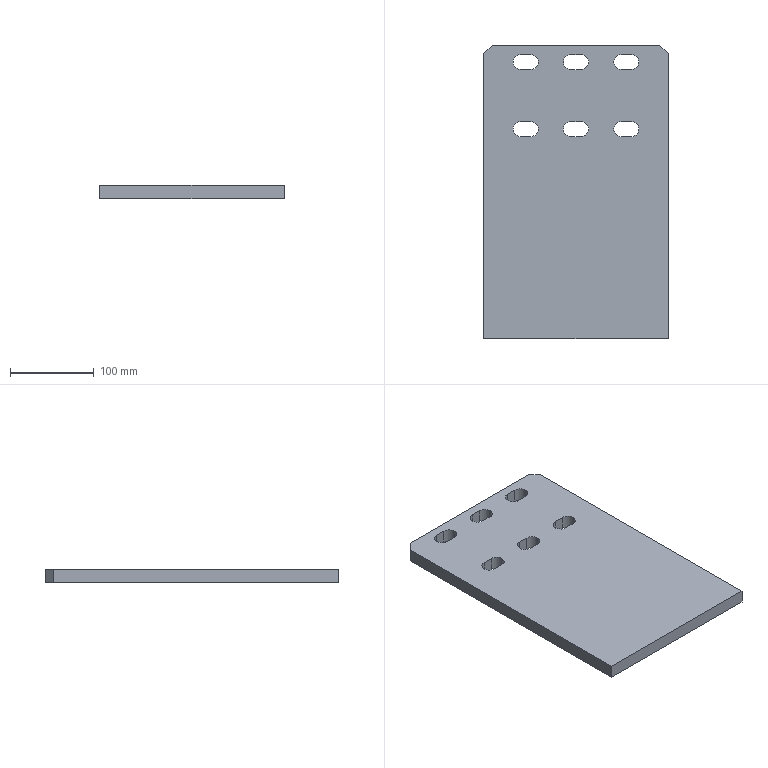Part | STEP file | VD-SYL0380DJ1006_1_1-11_VD-SYL0 | 1 solid | 38 faces | box 220 x 350 x 16 mm | volume 1185235 mm3 | plane 20 | cylinder 18 | commonest cylinder face diameters 18 x18
STEP:
#1=CARTESIAN_POINT('',(66.,66.,0.));
#2=VERTEX_POINT('',#1);
#3=CARTESIAN_POINT('',(75.,75.,0.));
#4=VERTEX_POINT('',#3);
#5=CARTESIAN_POINT('',(66.,75.,0.));
#6=DIRECTION('',(0.,0.,1.));
#7=DIRECTION('',(0.,-1.,0.));
#8=AXIS2_PLACEMENT_3D('',#5,#6,#7);
#9=CIRCLE('',#8,9.);
#10=EDGE_CURVE('',#2,#4,#9,.T.);
#11=ORIENTED_EDGE('',*,*,#10,.F.);
#12=CARTESIAN_POINT('',(66.,66.,16.));
#13=VERTEX_POINT('',#12);
#14=CARTESIAN_POINT('',(66.,66.,0.));
#15=DIRECTION('',(0.,0.,1.));
#16=VECTOR('',#15,1000.);
#17=LINE('',#14,#16);
#18=EDGE_CURVE('',#2,#13,#17,.T.);
#19=ORIENTED_EDGE('',*,*,#18,.T.);
#20=CARTESIAN_POINT('',(75.,75.,16.));
#21=VERTEX_POINT('',#20);
#22=CARTESIAN_POINT('',(66.,75.,16.));
#23=DIRECTION('',(0.,0.,-1.));
#24=DIRECTION('',(1.,0.,0.));
#25=AXIS2_PLACEMENT_3D('',#22,#23,#24);
#26=CIRCLE('',#25,9.);
#27=EDGE_CURVE('',#21,#13,#26,.T.);
#28=ORIENTED_EDGE('',*,*,#27,.F.);
#29=CARTESIAN_POINT('',(75.,75.,16.));
#30=DIRECTION('',(0.,0.,-1.));
#31=VECTOR('',#30,1000.);
#32=LINE('',#29,#31);
#33=EDGE_CURVE('',#21,#4,#32,.T.);
#34=ORIENTED_EDGE('',*,*,#33,.T.);
#35=EDGE_LOOP('',(#11,#19,#28,#34));
#36=FACE_OUTER_BOUND('',#35,.T.);
#37=CARTESIAN_POINT('',(66.,75.,8.));
#38=DIRECTION('',(0.,0.,1.));
#39=DIRECTION('',(1.,0.,0.));
#40=AXIS2_PLACEMENT_3D('',#37,#38,#39);
#41=CYLINDRICAL_SURFACE('',#40,9.);
#42=ADVANCED_FACE('',(#36),#41,.F.);
#43=ORIENTED_EDGE('',*,*,#33,.F.);
#44=CARTESIAN_POINT('',(66.,84.,16.));
#45=VERTEX_POINT('',#44);
#46=CARTESIAN_POINT('',(66.,75.,16.));
#47=DIRECTION('',(0.,0.,-1.));
#48=DIRECTION('',(0.,1.,0.));
#49=AXIS2_PLACEMENT_3D('',#46,#47,#48);
#50=CIRCLE('',#49,9.);
#51=EDGE_CURVE('',#45,#21,#50,.T.);
#52=ORIENTED_EDGE('',*,*,#51,.F.);
#53=CARTESIAN_POINT('',(66.,84.,0.));
#54=VERTEX_POINT('',#53);
#55=CARTESIAN_POINT('',(66.,84.,16.));
#56=DIRECTION('',(0.,0.,-1.));
#57=VECTOR('',#56,1000.);
#58=LINE('',#55,#57);
#59=EDGE_CURVE('',#45,#54,#58,.T.);
#60=ORIENTED_EDGE('',*,*,#59,.T.);
#61=CARTESIAN_POINT('',(66.,75.,0.));
#62=DIRECTION('',(0.,0.,1.));
#63=DIRECTION('',(1.,0.,0.));
#64=AXIS2_PLACEMENT_3D('',#61,#62,#63);
#65=CIRCLE('',#64,9.);
#66=EDGE_CURVE('',#4,#54,#65,.T.);
#67=ORIENTED_EDGE('',*,*,#66,.F.);
#68=EDGE_LOOP('',(#43,#52,#60,#67));
#69=FACE_OUTER_BOUND('',#68,.T.);
#70=CARTESIAN_POINT('',(66.,75.,8.));
#71=DIRECTION('',(0.,0.,1.));
#72=DIRECTION('',(1.,0.,0.));
#73=AXIS2_PLACEMENT_3D('',#70,#71,#72);
#74=CYLINDRICAL_SURFACE('',#73,9.);
#75=ADVANCED_FACE('',(#69),#74,.F.);
#76=CARTESIAN_POINT('',(54.,84.,0.));
#77=VERTEX_POINT('',#76);
#78=CARTESIAN_POINT('',(54.,84.,16.));
#79=VERTEX_POINT('',#78);
#80=CARTESIAN_POINT('',(54.,84.,0.));
#81=DIRECTION('',(0.,0.,1.));
#82=VECTOR('',#81,1000.);
#83=LINE('',#80,#82);
#84=EDGE_CURVE('',#77,#79,#83,.T.);
#85=ORIENTED_EDGE('',*,*,#84,.F.);
#86=CARTESIAN_POINT('',(66.,84.,0.));
#87=DIRECTION('',(-1.,0.,0.));
#88=VECTOR('',#87,1000.);
#89=LINE('',#86,#88);
#90=EDGE_CURVE('',#54,#77,#89,.T.);
#91=ORIENTED_EDGE('',*,*,#90,.F.);
#92=ORIENTED_EDGE('',*,*,#59,.F.);
#93=CARTESIAN_POINT('',(66.,84.,16.));
#94=DIRECTION('',(-1.,0.,0.));
#95=VECTOR('',#94,1000.);
#96=LINE('',#93,#95);
#97=EDGE_CURVE('',#45,#79,#96,.T.);
#98=ORIENTED_EDGE('',*,*,#97,.T.);
#99=EDGE_LOOP('',(#85,#91,#92,#98));
#100=FACE_OUTER_BOUND('',#99,.T.);
#101=CARTESIAN_POINT('',(63.,84.,8.));
#102=DIRECTION('',(0.,1.,0.));
#103=DIRECTION('',(1.,0.,0.));
#104=AXIS2_PLACEMENT_3D('',#101,#102,#103);
#105=PLANE('',#104);
#106=ADVANCED_FACE('',(#100),#105,.F.);
#107=CARTESIAN_POINT('',(54.,66.,16.));
#108=VERTEX_POINT('',#107);
#109=CARTESIAN_POINT('',(54.,75.,16.));
#110=DIRECTION('',(0.,0.,-1.));
#111=DIRECTION('',(-1.,0.,0.));
#112=AXIS2_PLACEMENT_3D('',#109,#110,#111);
#113=CIRCLE('',#112,9.);
#114=EDGE_CURVE('',#108,#79,#113,.T.);
#115=ORIENTED_EDGE('',*,*,#114,.F.);
#116=CARTESIAN_POINT('',(54.,66.,0.));
#117=VERTEX_POINT('',#116);
#118=CARTESIAN_POINT('',(54.,66.,16.));
#119=DIRECTION('',(0.,0.,-1.));
#120=VECTOR('',#119,1000.);
#121=LINE('',#118,#120);
#122=EDGE_CURVE('',#108,#117,#121,.T.);
#123=ORIENTED_EDGE('',*,*,#122,.T.);
#124=CARTESIAN_POINT('',(54.,75.,0.));
#125=DIRECTION('',(0.,0.,1.));
#126=DIRECTION('',(0.,1.,0.));
#127=AXIS2_PLACEMENT_3D('',#124,#125,#126);
#128=CIRCLE('',#127,9.);
#129=EDGE_CURVE('',#77,#117,#128,.T.);
#130=ORIENTED_EDGE('',*,*,#129,.F.);
#131=ORIENTED_EDGE('',*,*,#84,.T.);
#132=EDGE_LOOP('',(#115,#123,#130,#131));
#133=FACE_OUTER_BOUND('',#132,.T.);
#134=CARTESIAN_POINT('',(54.,75.,8.));
#135=DIRECTION('',(0.,0.,1.));
#136=DIRECTION('',(1.,0.,0.));
#137=AXIS2_PLACEMENT_3D('',#134,#135,#136);
#138=CYLINDRICAL_SURFACE('',#137,9.);
#139=ADVANCED_FACE('',(#133),#138,.F.);
#140=ORIENTED_EDGE('',*,*,#18,.F.);
#141=CARTESIAN_POINT('',(54.,66.,0.));
#142=DIRECTION('',(1.,0.,0.));
#143=VECTOR('',#142,1000.);
#144=LINE('',#141,#143);
#145=EDGE_CURVE('',#117,#2,#144,.T.);
#146=ORIENTED_EDGE('',*,*,#145,.F.);
#147=ORIENTED_EDGE('',*,*,#122,.F.);
#148=CARTESIAN_POINT('',(54.,66.,16.));
#149=DIRECTION('',(1.,0.,0.));
#150=VECTOR('',#149,1000.);
#151=LINE('',#148,#150);
#152=EDGE_CURVE('',#108,#13,#151,.T.);
#153=ORIENTED_EDGE('',*,*,#152,.T.);
#154=EDGE_LOOP('',(#140,#146,#147,#153));
#155=FACE_OUTER_BOUND('',#154,.T.);
#156=CARTESIAN_POINT('',(57.,66.,8.));
#157=DIRECTION('',(0.,-1.,0.));
#158=DIRECTION('',(0.,0.,-1.));
#159=AXIS2_PLACEMENT_3D('',#156,#157,#158);
#160=PLANE('',#159);
#161=ADVANCED_FACE('',(#155),#160,.F.);
#162=CARTESIAN_POINT('',(-6.,84.,0.));
#163=VERTEX_POINT('',#162);
#164=CARTESIAN_POINT('',(-6.,84.,16.));
#165=VERTEX_POINT('',#164);
#166=CARTESIAN_POINT('',(-6.,84.,0.));
#167=DIRECTION('',(0.,0.,1.));
#168=VECTOR('',#167,1000.);
#169=LINE('',#166,#168);
#170=EDGE_CURVE('',#163,#165,#169,.T.);
#171=ORIENTED_EDGE('',*,*,#170,.F.);
#172=CARTESIAN_POINT('',(6.,84.,0.));
#173=VERTEX_POINT('',#172);
#174=CARTESIAN_POINT('',(6.,84.,0.));
#175=DIRECTION('',(-1.,0.,0.));
#176=VECTOR('',#175,1000.);
#177=LINE('',#174,#176);
#178=EDGE_CURVE('',#173,#163,#177,.T.);
#179=ORIENTED_EDGE('',*,*,#178,.F.);
#180=CARTESIAN_POINT('',(6.,84.,16.));
#181=VERTEX_POINT('',#180);
#182=CARTESIAN_POINT('',(6.,84.,16.));
#183=DIRECTION('',(0.,0.,-1.));
#184=VECTOR('',#183,1000.);
#185=LINE('',#182,#184);
#186=EDGE_CURVE('',#181,#173,#185,.T.);
#187=ORIENTED_EDGE('',*,*,#186,.F.);
#188=CARTESIAN_POINT('',(6.,84.,16.));
#189=DIRECTION('',(-1.,0.,0.));
#190=VECTOR('',#189,1000.);
#191=LINE('',#188,#190);
#192=EDGE_CURVE('',#181,#165,#191,.T.);
#193=ORIENTED_EDGE('',*,*,#192,.T.);
#194=EDGE_LOOP('',(#171,#179,#187,#193));
#195=FACE_OUTER_BOUND('',#194,.T.);
#196=CARTESIAN_POINT('',(3.,84.,8.));
#197=DIRECTION('',(0.,1.,0.));
#198=DIRECTION('',(1.,0.,0.));
#199=AXIS2_PLACEMENT_3D('',#196,#197,#198);
#200=PLANE('',#199);
#201=ADVANCED_FACE('',(#195),#200,.F.);
#202=CARTESIAN_POINT('',(15.,75.,16.));
#203=VERTEX_POINT('',#202);
#204=CARTESIAN_POINT('',(15.,75.,0.));
#205=VERTEX_POINT('',#204);
#206=CARTESIAN_POINT('',(15.,75.,16.));
#207=DIRECTION('',(0.,0.,-1.));
#208=VECTOR('',#207,1000.);
#209=LINE('',#206,#208);
#210=EDGE_CURVE('',#203,#205,#209,.T.);
#211=ORIENTED_EDGE('',*,*,#210,.F.);
#212=CARTESIAN_POINT('',(6.,75.,16.));
#213=DIRECTION('',(0.,0.,-1.));
#214=DIRECTION('',(0.,1.,0.));
#215=AXIS2_PLACEMENT_3D('',#212,#213,#214);
#216=CIRCLE('',#215,9.);
#217=EDGE_CURVE('',#181,#203,#216,.T.);
#218=ORIENTED_EDGE('',*,*,#217,.F.);
#219=ORIENTED_EDGE('',*,*,#186,.T.);
#220=CARTESIAN_POINT('',(6.,75.,0.));
#221=DIRECTION('',(0.,0.,1.));
#222=DIRECTION('',(1.,0.,0.));
#223=AXIS2_PLACEMENT_3D('',#220,#221,#222);
#224=CIRCLE('',#223,9.);
#225=EDGE_CURVE('',#205,#173,#224,.T.);
#226=ORIENTED_EDGE('',*,*,#225,.F.);
#227=EDGE_LOOP('',(#211,#218,#219,#226));
#228=FACE_OUTER_BOUND('',#227,.T.);
#229=CARTESIAN_POINT('',(6.,75.,8.));
#230=DIRECTION('',(0.,0.,1.));
#231=DIRECTION('',(1.,0.,0.));
#232=AXIS2_PLACEMENT_3D('',#229,#230,#231);
#233=CYLINDRICAL_SURFACE('',#232,9.);
#234=ADVANCED_FACE('',(#228),#233,.F.);
#235=CARTESIAN_POINT('',(6.,66.,0.));
#236=VERTEX_POINT('',#235);
#237=CARTESIAN_POINT('',(6.,75.,0.));
#238=DIRECTION('',(0.,0.,1.));
#239=DIRECTION('',(0.,-1.,0.));
#240=AXIS2_PLACEMENT_3D('',#237,#238,#239);
#241=CIRCLE('',#240,9.);
#242=EDGE_CURVE('',#236,#205,#241,.T.);
#243=ORIENTED_EDGE('',*,*,#242,.F.);
#244=CARTESIAN_POINT('',(6.,66.,16.));
#245=VERTEX_POINT('',#244);
#246=CARTESIAN_POINT('',(6.,66.,0.));
#247=DIRECTION('',(0.,0.,1.));
#248=VECTOR('',#247,1000.);
#249=LINE('',#246,#248);
#250=EDGE_CURVE('',#236,#245,#249,.T.);
#251=ORIENTED_EDGE('',*,*,#250,.T.);
#252=CARTESIAN_POINT('',(6.,75.,16.));
#253=DIRECTION('',(0.,0.,-1.));
#254=DIRECTION('',(1.,0.,0.));
#255=AXIS2_PLACEMENT_3D('',#252,#253,#254);
#256=CIRCLE('',#255,9.);
#257=EDGE_CURVE('',#203,#245,#256,.T.);
#258=ORIENTED_EDGE('',*,*,#257,.F.);
#259=ORIENTED_EDGE('',*,*,#210,.T.);
#260=EDGE_LOOP('',(#243,#251,#258,#259));
#261=FACE_OUTER_BOUND('',#260,.T.);
#262=CARTESIAN_POINT('',(6.,75.,8.));
#263=DIRECTION('',(0.,0.,1.));
#264=DIRECTION('',(1.,0.,0.));
#265=AXIS2_PLACEMENT_3D('',#262,#263,#264);
#266=CYLINDRICAL_SURFACE('',#265,9.);
#267=ADVANCED_FACE('',(#261),#266,.F.);
#268=ORIENTED_EDGE('',*,*,#250,.F.);
#269=CARTESIAN_POINT('',(-6.,66.,0.));
#270=VERTEX_POINT('',#269);
#271=CARTESIAN_POINT('',(-6.,66.,0.));
#272=DIRECTION('',(1.,0.,0.));
#273=VECTOR('',#272,1000.);
#274=LINE('',#271,#273);
#275=EDGE_CURVE('',#270,#236,#274,.T.);
#276=ORIENTED_EDGE('',*,*,#275,.F.);
#277=CARTESIAN_POINT('',(-6.,66.,16.));
#278=VERTEX_POINT('',#277);
#279=CARTESIAN_POINT('',(-6.,66.,16.));
#280=DIRECTION('',(0.,0.,-1.));
#281=VECTOR('',#280,1000.);
#282=LINE('',#279,#281);
#283=EDGE_CURVE('',#278,#270,#282,.T.);
#284=ORIENTED_EDGE('',*,*,#283,.F.);
#285=CARTESIAN_POINT('',(-6.,66.,16.));
#286=DIRECTION('',(1.,0.,0.));
#287=VECTOR('',#286,1000.);
#288=LINE('',#285,#287);
#289=EDGE_CURVE('',#278,#245,#288,.T.);
#290=ORIENTED_EDGE('',*,*,#289,.T.);
#291=EDGE_LOOP('',(#268,#276,#284,#290));
#292=FACE_OUTER_BOUND('',#291,.T.);
#293=CARTESIAN_POINT('',(-3.,66.,8.));
#294=DIRECTION('',(0.,-1.,0.));
#295=DIRECTION('',(0.,0.,-1.));
#296=AXIS2_PLACEMENT_3D('',#293,#294,#295);
#297=PLANE('',#296);
#298=ADVANCED_FACE('',(#292),#297,.F.);
#299=CARTESIAN_POINT('',(-54.,66.,0.));
#300=VERTEX_POINT('',#299);
#301=CARTESIAN_POINT('',(-45.,75.,0.));
#302=VERTEX_POINT('',#301);
#303=CARTESIAN_POINT('',(-54.,75.,0.));
#304=DIRECTION('',(0.,0.,1.));
#305=DIRECTION('',(0.,-1.,0.));
#306=AXIS2_PLACEMENT_3D('',#303,#304,#305);
#307=CIRCLE('',#306,9.);
#308=EDGE_CURVE('',#300,#302,#307,.T.);
#309=ORIENTED_EDGE('',*,*,#308,.F.);
#310=CARTESIAN_POINT('',(-54.,66.,16.));
#311=VERTEX_POINT('',#310);
#312=CARTESIAN_POINT('',(-54.,66.,0.));
#313=DIRECTION('',(0.,0.,1.));
#314=VECTOR('',#313,1000.);
#315=LINE('',#312,#314);
#316=EDGE_CURVE('',#300,#311,#315,.T.);
#317=ORIENTED_EDGE('',*,*,#316,.T.);
#318=CARTESIAN_POINT('',(-45.,75.,16.));
#319=VERTEX_POINT('',#318);
#320=CARTESIAN_POINT('',(-54.,75.,16.));
#321=DIRECTION('',(0.,0.,-1.));
#322=DIRECTION('',(1.,0.,0.));
#323=AXIS2_PLACEMENT_3D('',#320,#321,#322);
#324=CIRCLE('',#323,9.);
#325=EDGE_CURVE('',#319,#311,#324,.T.);
#326=ORIENTED_EDGE('',*,*,#325,.F.);
#327=CARTESIAN_POINT('',(-45.,75.,16.));
#328=DIRECTION('',(0.,0.,-1.));
#329=VECTOR('',#328,1000.);
#330=LINE('',#327,#329);
#331=EDGE_CURVE('',#319,#302,#330,.T.);
#332=ORIENTED_EDGE('',*,*,#331,.T.);
#333=EDGE_LOOP('',(#309,#317,#326,#332));
#334=FACE_OUTER_BOUND('',#333,.T.);
#335=CARTESIAN_POINT('',(-54.,75.,8.));
#336=DIRECTION('',(0.,0.,1.));
#337=DIRECTION('',(1.,0.,0.));
#338=AXIS2_PLACEMENT_3D('',#335,#336,#337);
#339=CYLINDRICAL_SURFACE('',#338,9.);
#340=ADVANCED_FACE('',(#334),#339,.F.);
#341=ORIENTED_EDGE('',*,*,#331,.F.);
#342=CARTESIAN_POINT('',(-54.,84.,16.));
#343=VERTEX_POINT('',#342);
#344=CARTESIAN_POINT('',(-54.,75.,16.));
#345=DIRECTION('',(0.,0.,-1.));
#346=DIRECTION('',(0.,1.,0.));
#347=AXIS2_PLACEMENT_3D('',#344,#345,#346);
#348=CIRCLE('',#347,9.);
#349=EDGE_CURVE('',#343,#319,#348,.T.);
#350=ORIENTED_EDGE('',*,*,#349,.F.);
#351=CARTESIAN_POINT('',(-54.,84.,0.));
#352=VERTEX_POINT('',#351);
#353=CARTESIAN_POINT('',(-54.,84.,16.));
#354=DIRECTION('',(0.,0.,-1.));
#355=VECTOR('',#354,1000.);
#356=LINE('',#353,#355);
#357=EDGE_CURVE('',#343,#352,#356,.T.);
#358=ORIENTED_EDGE('',*,*,#357,.T.);
#359=CARTESIAN_POINT('',(-54.,75.,0.));
#360=DIRECTION('',(0.,0.,1.));
#361=DIRECTION('',(1.,0.,0.));
#362=AXIS2_PLACEMENT_3D('',#359,#360,#361);
#363=CIRCLE('',#362,9.);
#364=EDGE_CURVE('',#302,#352,#363,.T.);
#365=ORIENTED_EDGE('',*,*,#364,.F.);
#366=EDGE_LOOP('',(#341,#350,#358,#365));
#367=FACE_OUTER_BOUND('',#366,.T.);
#368=CARTESIAN_POINT('',(-54.,75.,8.));
#369=DIRECTION('',(0.,0.,1.));
#370=DIRECTION('',(1.,0.,0.));
#371=AXIS2_PLACEMENT_3D('',#368,#369,#370);
#372=CYLINDRICAL_SURFACE('',#371,9.);
#373=ADVANCED_FACE('',(#367),#372,.F.);
#374=CARTESIAN_POINT('',(-66.,84.,0.));
#375=VERTEX_POINT('',#374);
#376=CARTESIAN_POINT('',(-66.,84.,16.));
#377=VERTEX_POINT('',#376);
#378=CARTESIAN_POINT('',(-66.,84.,0.));
#379=DIRECTION('',(0.,0.,1.));
#380=VECTOR('',#379,1000.);
#381=LINE('',#378,#380);
#382=EDGE_CURVE('',#375,#377,#381,.T.);
#383=ORIENTED_EDGE('',*,*,#382,.F.);
#384=CARTESIAN_POINT('',(-54.,84.,0.));
#385=DIRECTION('',(-1.,0.,0.));
#386=VECTOR('',#385,1000.);
#387=LINE('',#384,#386);
#388=EDGE_CURVE('',#352,#375,#387,.T.);
#389=ORIENTED_EDGE('',*,*,#388,.F.);
#390=ORIENTED_EDGE('',*,*,#357,.F.);
#391=CARTESIAN_POINT('',(-54.,84.,16.));
#392=DIRECTION('',(-1.,0.,0.));
#393=VECTOR('',#392,1000.);
#394=LINE('',#391,#393);
#395=EDGE_CURVE('',#343,#377,#394,.T.);
#396=ORIENTED_EDGE('',*,*,#395,.T.);
#397=EDGE_LOOP('',(#383,#389,#390,#396));
#398=FACE_OUTER_BOUND('',#397,.T.);
#399=CARTESIAN_POINT('',(-57.,84.,8.));
#400=DIRECTION('',(0.,1.,0.));
#401=DIRECTION('',(1.,0.,0.));
#402=AXIS2_PLACEMENT_3D('',#399,#400,#401);
#403=PLANE('',#402);
#404=ADVANCED_FACE('',(#398),#403,.F.);
#405=CARTESIAN_POINT('',(-66.,66.,16.));
#406=VERTEX_POINT('',#405);
#407=CARTESIAN_POINT('',(-66.,75.,16.));
#408=DIRECTION('',(0.,0.,-1.));
#409=DIRECTION('',(-1.,0.,0.));
#410=AXIS2_PLACEMENT_3D('',#407,#408,#409);
#411=CIRCLE('',#410,9.);
#412=EDGE_CURVE('',#406,#377,#411,.T.);
#413=ORIENTED_EDGE('',*,*,#412,.F.);
#414=CARTESIAN_POINT('',(-66.,66.,0.));
#415=VERTEX_POINT('',#414);
#416=CARTESIAN_POINT('',(-66.,66.,16.));
#417=DIRECTION('',(0.,0.,-1.));
#418=VECTOR('',#417,1000.);
#419=LINE('',#416,#418);
#420=EDGE_CURVE('',#406,#415,#419,.T.);
#421=ORIENTED_EDGE('',*,*,#420,.T.);
#422=CARTESIAN_POINT('',(-66.,75.,0.));
#423=DIRECTION('',(0.,0.,1.));
#424=DIRECTION('',(0.,1.,0.));
#425=AXIS2_PLACEMENT_3D('',#422,#423,#424);
#426=CIRCLE('',#425,9.);
#427=EDGE_CURVE('',#375,#415,#426,.T.);
#428=ORIENTED_EDGE('',*,*,#427,.F.);
#429=ORIENTED_EDGE('',*,*,#382,.T.);
#430=EDGE_LOOP('',(#413,#421,#428,#429));
#431=FACE_OUTER_BOUND('',#430,.T.);
#432=CARTESIAN_POINT('',(-66.,75.,8.));
#433=DIRECTION('',(0.,0.,1.));
#434=DIRECTION('',(1.,0.,0.));
#435=AXIS2_PLACEMENT_3D('',#432,#433,#434);
#436=CYLINDRICAL_SURFACE('',#435,9.);
#437=ADVANCED_FACE('',(#431),#436,.F.);
#438=ORIENTED_EDGE('',*,*,#316,.F.);
#439=CARTESIAN_POINT('',(-66.,66.,0.));
#440=DIRECTION('',(1.,0.,0.));
#441=VECTOR('',#440,1000.);
#442=LINE('',#439,#441);
#443=EDGE_CURVE('',#415,#300,#442,.T.);
#444=ORIENTED_EDGE('',*,*,#443,.F.);
#445=ORIENTED_EDGE('',*,*,#420,.F.);
#446=CARTESIAN_POINT('',(-66.,66.,16.));
#447=DIRECTION('',(1.,0.,0.));
#448=VECTOR('',#447,1000.);
#449=LINE('',#446,#448);
#450=EDGE_CURVE('',#406,#311,#449,.T.);
#451=ORIENTED_EDGE('',*,*,#450,.T.);
#452=EDGE_LOOP('',(#438,#444,#445,#451));
#453=FACE_OUTER_BOUND('',#452,.T.);
#454=CARTESIAN_POINT('',(-63.,66.,8.));
#455=DIRECTION('',(0.,-1.,0.));
#456=DIRECTION('',(0.,0.,-1.));
#457=AXIS2_PLACEMENT_3D('',#454,#455,#456);
#458=PLANE('',#457);
#459=ADVANCED_FACE('',(#453),#458,.F.);
#460=CARTESIAN_POINT('',(66.,146.,0.));
#461=VERTEX_POINT('',#460);
#462=CARTESIAN_POINT('',(75.,155.,0.));
#463=VERTEX_POINT('',#462);
#464=CARTESIAN_POINT('',(66.,155.,0.));
#465=DIRECTION('',(0.,0.,1.));
#466=DIRECTION('',(0.,-1.,0.));
#467=AXIS2_PLACEMENT_3D('',#464,#465,#466);
#468=CIRCLE('',#467,9.);
#469=EDGE_CURVE('',#461,#463,#468,.T.);
#470=ORIENTED_EDGE('',*,*,#469,.F.);
#471=CARTESIAN_POINT('',(66.,146.,16.));
#472=VERTEX_POINT('',#471);
#473=CARTESIAN_POINT('',(66.,146.,0.));
#474=DIRECTION('',(0.,0.,1.));
#475=VECTOR('',#474,1000.);
#476=LINE('',#473,#475);
#477=EDGE_CURVE('',#461,#472,#476,.T.);
#478=ORIENTED_EDGE('',*,*,#477,.T.);
#479=CARTESIAN_POINT('',(75.,155.,16.));
#480=VERTEX_POINT('',#479);
#481=CARTESIAN_POINT('',(66.,155.,16.));
#482=DIRECTION('',(0.,0.,-1.));
#483=DIRECTION('',(1.,0.,0.));
#484=AXIS2_PLACEMENT_3D('',#481,#482,#483);
#485=CIRCLE('',#484,9.);
#486=EDGE_CURVE('',#480,#472,#485,.T.);
#487=ORIENTED_EDGE('',*,*,#486,.F.);
#488=CARTESIAN_POINT('',(75.,155.,16.));
#489=DIRECTION('',(0.,0.,-1.));
#490=VECTOR('',#489,1000.);
#491=LINE('',#488,#490);
#492=EDGE_CURVE('',#480,#463,#491,.T.);
#493=ORIENTED_EDGE('',*,*,#492,.T.);
#494=EDGE_LOOP('',(#470,#478,#487,#493));
#495=FACE_OUTER_BOUND('',#494,.T.);
#496=CARTESIAN_POINT('',(66.,155.,8.));
#497=DIRECTION('',(0.,0.,1.));
#498=DIRECTION('',(1.,0.,0.));
#499=AXIS2_PLACEMENT_3D('',#496,#497,#498);
#500=CYLINDRICAL_SURFACE('',#499,9.);
#501=ADVANCED_FACE('',(#495),#500,.F.);
#502=ORIENTED_EDGE('',*,*,#492,.F.);
#503=CARTESIAN_POINT('',(66.,164.,16.));
#504=VERTEX_POINT('',#503);
#505=CARTESIAN_POINT('',(66.,155.,16.));
#506=DIRECTION('',(0.,0.,-1.));
#507=DIRECTION('',(0.,1.,0.));
#508=AXIS2_PLACEMENT_3D('',#505,#506,#507);
#509=CIRCLE('',#508,9.);
#510=EDGE_CURVE('',#504,#480,#509,.T.);
#511=ORIENTED_EDGE('',*,*,#510,.F.);
#512=CARTESIAN_POINT('',(66.,164.,0.));
#513=VERTEX_POINT('',#512);
#514=CARTESIAN_POINT('',(66.,164.,16.));
#515=DIRECTION('',(0.,0.,-1.));
#516=VECTOR('',#515,1000.);
#517=LINE('',#514,#516);
#518=EDGE_CURVE('',#504,#513,#517,.T.);
#519=ORIENTED_EDGE('',*,*,#518,.T.);
#520=CARTESIAN_POINT('',(66.,155.,0.));
#521=DIRECTION('',(0.,0.,1.));
#522=DIRECTION('',(1.,0.,0.));
#523=AXIS2_PLACEMENT_3D('',#520,#521,#522);
#524=CIRCLE('',#523,9.);
#525=EDGE_CURVE('',#463,#513,#524,.T.);
#526=ORIENTED_EDGE('',*,*,#525,.F.);
#527=EDGE_LOOP('',(#502,#511,#519,#526));
#528=FACE_OUTER_BOUND('',#527,.T.);
#529=CARTESIAN_POINT('',(66.,155.,8.));
#530=DIRECTION('',(0.,0.,1.));
#531=DIRECTION('',(1.,0.,0.));
#532=AXIS2_PLACEMENT_3D('',#529,#530,#531);
#533=CYLINDRICAL_SURFACE('',#532,9.);
#534=ADVANCED_FACE('',(#528),#533,.F.);
#535=CARTESIAN_POINT('',(54.,164.,0.));
#536=VERTEX_POINT('',#535);
#537=CARTESIAN_POINT('',(54.,164.,16.));
#538=VERTEX_POINT('',#537);
#539=CARTESIAN_POINT('',(54.,164.,0.));
#540=DIRECTION('',(0.,0.,1.));
#541=VECTOR('',#540,1000.);
#542=LINE('',#539,#541);
#543=EDGE_CURVE('',#536,#538,#542,.T.);
#544=ORIENTED_EDGE('',*,*,#543,.F.);
#545=CARTESIAN_POINT('',(66.,164.,0.));
#546=DIRECTION('',(-1.,0.,0.));
#547=VECTOR('',#546,1000.);
#548=LINE('',#545,#547);
#549=EDGE_CURVE('',#513,#536,#548,.T.);
#550=ORIENTED_EDGE('',*,*,#549,.F.);
#551=ORIENTED_EDGE('',*,*,#518,.F.);
#552=CARTESIAN_POINT('',(66.,164.,16.));
#553=DIRECTION('',(-1.,0.,0.));
#554=VECTOR('',#553,1000.);
#555=LINE('',#552,#554);
#556=EDGE_CURVE('',#504,#538,#555,.T.);
#557=ORIENTED_EDGE('',*,*,#556,.T.);
#558=EDGE_LOOP('',(#544,#550,#551,#557));
#559=FACE_OUTER_BOUND('',#558,.T.);
#560=CARTESIAN_POINT('',(63.,164.,8.));
#561=DIRECTION('',(0.,1.,0.));
#562=DIRECTION('',(1.,0.,0.));
#563=AXIS2_PLACEMENT_3D('',#560,#561,#562);
#564=PLANE('',#563);
#565=ADVANCED_FACE('',(#559),#564,.F.);
#566=CARTESIAN_POINT('',(54.,146.,16.));
#567=VERTEX_POINT('',#566);
#568=CARTESIAN_POINT('',(54.,155.,16.));
#569=DIRECTION('',(0.,0.,-1.));
#570=DIRECTION('',(-1.,0.,0.));
#571=AXIS2_PLACEMENT_3D('',#568,#569,#570);
#572=CIRCLE('',#571,9.);
#573=EDGE_CURVE('',#567,#538,#572,.T.);
#574=ORIENTED_EDGE('',*,*,#573,.F.);
#575=CARTESIAN_POINT('',(54.,146.,0.));
#576=VERTEX_POINT('',#575);
#577=CARTESIAN_POINT('',(54.,146.,16.));
#578=DIRECTION('',(0.,0.,-1.));
#579=VECTOR('',#578,1000.);
#580=LINE('',#577,#579);
#581=EDGE_CURVE('',#567,#576,#580,.T.);
#582=ORIENTED_EDGE('',*,*,#581,.T.);
#583=CARTESIAN_POINT('',(54.,155.,0.));
#584=DIRECTION('',(0.,0.,1.));
#585=DIRECTION('',(0.,1.,0.));
#586=AXIS2_PLACEMENT_3D('',#583,#584,#585);
#587=CIRCLE('',#586,9.);
#588=EDGE_CURVE('',#536,#576,#587,.T.);
#589=ORIENTED_EDGE('',*,*,#588,.F.);
#590=ORIENTED_EDGE('',*,*,#543,.T.);
#591=EDGE_LOOP('',(#574,#582,#589,#590));
#592=FACE_OUTER_BOUND('',#591,.T.);
#593=CARTESIAN_POINT('',(54.,155.,8.));
#594=DIRECTION('',(0.,0.,1.));
#595=DIRECTION('',(1.,0.,0.));
#596=AXIS2_PLACEMENT_3D('',#593,#594,#595);
#597=CYLINDRICAL_SURFACE('',#596,9.);
#598=ADVANCED_FACE('',(#592),#597,.F.);
#599=ORIENTED_EDGE('',*,*,#477,.F.);
#600=CARTESIAN_POINT('',(54.,146.,0.));
#601=DIRECTION('',(1.,0.,0.));
#602=VECTOR('',#601,1000.);
#603=LINE('',#600,#602);
#604=EDGE_CURVE('',#576,#461,#603,.T.);
#605=ORIENTED_EDGE('',*,*,#604,.F.);
#606=ORIENTED_EDGE('',*,*,#581,.F.);
#607=CARTESIAN_POINT('',(54.,146.,16.));
#608=DIRECTION('',(1.,0.,0.));
#609=VECTOR('',#608,1000.);
#610=LINE('',#607,#609);
#611=EDGE_CURVE('',#567,#472,#610,.T.);
#612=ORIENTED_EDGE('',*,*,#611,.T.);
#613=EDGE_LOOP('',(#599,#605,#606,#612));
#614=FACE_OUTER_BOUND('',#613,.T.);
#615=CARTESIAN_POINT('',(57.,146.,8.));
#616=DIRECTION('',(0.,-1.,0.));
#617=DIRECTION('',(0.,0.,-1.));
#618=AXIS2_PLACEMENT_3D('',#615,#616,#617);
#619=PLANE('',#618);
#620=ADVANCED_FACE('',(#614),#619,.F.);
#621=CARTESIAN_POINT('',(6.,146.,0.));
#622=VERTEX_POINT('',#621);
#623=CARTESIAN_POINT('',(15.,155.,0.));
#624=VERTEX_POINT('',#623);
#625=CARTESIAN_POINT('',(6.,155.,0.));
#626=DIRECTION('',(0.,0.,1.));
#627=DIRECTION('',(0.,-1.,0.));
#628=AXIS2_PLACEMENT_3D('',#625,#626,#627);
#629=CIRCLE('',#628,9.);
#630=EDGE_CURVE('',#622,#624,#629,.T.);
#631=ORIENTED_EDGE('',*,*,#630,.F.);
#632=CARTESIAN_POINT('',(6.,146.,16.));
#633=VERTEX_POINT('',#632);
#634=CARTESIAN_POINT('',(6.,146.,0.));
#635=DIRECTION('',(0.,0.,1.));
#636=VECTOR('',#635,1000.);
#637=LINE('',#634,#636);
#638=EDGE_CURVE('',#622,#633,#637,.T.);
#639=ORIENTED_EDGE('',*,*,#638,.T.);
#640=CARTESIAN_POINT('',(15.,155.,16.));
#641=VERTEX_POINT('',#640);
#642=CARTESIAN_POINT('',(6.,155.,16.));
#643=DIRECTION('',(0.,0.,-1.));
#644=DIRECTION('',(1.,0.,0.));
#645=AXIS2_PLACEMENT_3D('',#642,#643,#644);
#646=CIRCLE('',#645,9.);
#647=EDGE_CURVE('',#641,#633,#646,.T.);
#648=ORIENTED_EDGE('',*,*,#647,.F.);
#649=CARTESIAN_POINT('',(15.,155.,16.));
#650=DIRECTION('',(0.,0.,-1.));
#651=VECTOR('',#650,1000.);
#652=LINE('',#649,#651);
#653=EDGE_CURVE('',#641,#624,#652,.T.);
#654=ORIENTED_EDGE('',*,*,#653,.T.);
#655=EDGE_LOOP('',(#631,#639,#648,#654));
#656=FACE_OUTER_BOUND('',#655,.T.);
#657=CARTESIAN_POINT('',(6.,155.,8.));
#658=DIRECTION('',(0.,0.,1.));
#659=DIRECTION('',(1.,0.,0.));
#660=AXIS2_PLACEMENT_3D('',#657,#658,#659);
#661=CYLINDRICAL_SURFACE('',#660,9.);
#662=ADVANCED_FACE('',(#656),#661,.F.);
#663=ORIENTED_EDGE('',*,*,#653,.F.);
#664=CARTESIAN_POINT('',(6.,164.,16.));
#665=VERTEX_POINT('',#664);
#666=CARTESIAN_POINT('',(6.,155.,16.));
#667=DIRECTION('',(0.,0.,-1.));
#668=DIRECTION('',(0.,1.,0.));
#669=AXIS2_PLACEMENT_3D('',#666,#667,#668);
#670=CIRCLE('',#669,9.);
#671=EDGE_CURVE('',#665,#641,#670,.T.);
#672=ORIENTED_EDGE('',*,*,#671,.F.);
#673=CARTESIAN_POINT('',(6.,164.,0.));
#674=VERTEX_POINT('',#673);
#675=CARTESIAN_POINT('',(6.,164.,16.));
#676=DIRECTION('',(0.,0.,-1.));
#677=VECTOR('',#676,1000.);
#678=LINE('',#675,#677);
#679=EDGE_CURVE('',#665,#674,#678,.T.);
#680=ORIENTED_EDGE('',*,*,#679,.T.);
#681=CARTESIAN_POINT('',(6.,155.,0.));
#682=DIRECTION('',(0.,0.,1.));
#683=DIRECTION('',(1.,0.,0.));
#684=AXIS2_PLACEMENT_3D('',#681,#682,#683);
#685=CIRCLE('',#684,9.);
#686=EDGE_CURVE('',#624,#674,#685,.T.);
#687=ORIENTED_EDGE('',*,*,#686,.F.);
#688=EDGE_LOOP('',(#663,#672,#680,#687));
#689=FACE_OUTER_BOUND('',#688,.T.);
#690=CARTESIAN_POINT('',(6.,155.,8.));
#691=DIRECTION('',(0.,0.,1.));
#692=DIRECTION('',(1.,0.,0.));
#693=AXIS2_PLACEMENT_3D('',#690,#691,#692);
#694=CYLINDRICAL_SURFACE('',#693,9.);
#695=ADVANCED_FACE('',(#689),#694,.F.);
#696=CARTESIAN_POINT('',(-6.,164.,0.));
#697=VERTEX_POINT('',#696);
#698=CARTESIAN_POINT('',(-6.,164.,16.));
#699=VERTEX_POINT('',#698);
#700=CARTESIAN_POINT('',(-6.,164.,0.));
#701=DIRECTION('',(0.,0.,1.));
#702=VECTOR('',#701,1000.);
#703=LINE('',#700,#702);
#704=EDGE_CURVE('',#697,#699,#703,.T.);
#705=ORIENTED_EDGE('',*,*,#704,.F.);
#706=CARTESIAN_POINT('',(6.,164.,0.));
#707=DIRECTION('',(-1.,0.,0.));
#708=VECTOR('',#707,1000.);
#709=LINE('',#706,#708);
#710=EDGE_CURVE('',#674,#697,#709,.T.);
#711=ORIENTED_EDGE('',*,*,#710,.F.);
#712=ORIENTED_EDGE('',*,*,#679,.F.);
#713=CARTESIAN_POINT('',(6.,164.,16.));
#714=DIRECTION('',(-1.,0.,0.));
#715=VECTOR('',#714,1000.);
#716=LINE('',#713,#715);
#717=EDGE_CURVE('',#665,#699,#716,.T.);
#718=ORIENTED_EDGE('',*,*,#717,.T.);
#719=EDGE_LOOP('',(#705,#711,#712,#718));
#720=FACE_OUTER_BOUND('',#719,.T.);
#721=CARTESIAN_POINT('',(3.,164.,8.));
#722=DIRECTION('',(0.,1.,0.));
#723=DIRECTION('',(1.,0.,0.));
#724=AXIS2_PLACEMENT_3D('',#721,#722,#723);
#725=PLANE('',#724);
#726=ADVANCED_FACE('',(#720),#725,.F.);
#727=CARTESIAN_POINT('',(-6.,146.,16.));
#728=VERTEX_POINT('',#727);
#729=CARTESIAN_POINT('',(-6.,155.,16.));
#730=DIRECTION('',(0.,0.,-1.));
#731=DIRECTION('',(-1.,0.,0.));
#732=AXIS2_PLACEMENT_3D('',#729,#730,#731);
#733=CIRCLE('',#732,9.);
#734=EDGE_CURVE('',#728,#699,#733,.T.);
#735=ORIENTED_EDGE('',*,*,#734,.F.);
#736=CARTESIAN_POINT('',(-6.,146.,0.));
#737=VERTEX_POINT('',#736);
#738=CARTESIAN_POINT('',(-6.,146.,16.));
#739=DIRECTION('',(0.,0.,-1.));
#740=VECTOR('',#739,1000.);
#741=LINE('',#738,#740);
#742=EDGE_CURVE('',#728,#737,#741,.T.);
#743=ORIENTED_EDGE('',*,*,#742,.T.);
#744=CARTESIAN_POINT('',(-6.,155.,0.));
#745=DIRECTION('',(0.,0.,1.));
#746=DIRECTION('',(0.,1.,0.));
#747=AXIS2_PLACEMENT_3D('',#744,#745,#746);
#748=CIRCLE('',#747,9.);
#749=EDGE_CURVE('',#697,#737,#748,.T.);
#750=ORIENTED_EDGE('',*,*,#749,.F.);
#751=ORIENTED_EDGE('',*,*,#704,.T.);
#752=EDGE_LOOP('',(#735,#743,#750,#751));
#753=FACE_OUTER_BOUND('',#752,.T.);
#754=CARTESIAN_POINT('',(-6.,155.,8.));
#755=DIRECTION('',(0.,0.,1.));
#756=DIRECTION('',(1.,0.,0.));
#757=AXIS2_PLACEMENT_3D('',#754,#755,#756);
#758=CYLINDRICAL_SURFACE('',#757,9.);
#759=ADVANCED_FACE('',(#753),#758,.F.);
#760=ORIENTED_EDGE('',*,*,#638,.F.);
#761=CARTESIAN_POINT('',(-6.,146.,0.));
#762=DIRECTION('',(1.,0.,0.));
#763=VECTOR('',#762,1000.);
#764=LINE('',#761,#763);
#765=EDGE_CURVE('',#737,#622,#764,.T.);
#766=ORIENTED_EDGE('',*,*,#765,.F.);
#767=ORIENTED_EDGE('',*,*,#742,.F.);
#768=CARTESIAN_POINT('',(-6.,146.,16.));
#769=DIRECTION('',(1.,0.,0.));
#770=VECTOR('',#769,1000.);
#771=LINE('',#768,#770);
#772=EDGE_CURVE('',#728,#633,#771,.T.);
#773=ORIENTED_EDGE('',*,*,#772,.T.);
#774=EDGE_LOOP('',(#760,#766,#767,#773));
#775=FACE_OUTER_BOUND('',#774,.T.);
#776=CARTESIAN_POINT('',(-3.,146.,8.));
#777=DIRECTION('',(0.,-1.,0.));
#778=DIRECTION('',(0.,0.,-1.));
#779=AXIS2_PLACEMENT_3D('',#776,#777,#778);
#780=PLANE('',#779);
#781=ADVANCED_FACE('',(#775),#780,.F.);
#782=CARTESIAN_POINT('',(-54.,146.,0.));
#783=VERTEX_POINT('',#782);
#784=CARTESIAN_POINT('',(-45.,155.,0.));
#785=VERTEX_POINT('',#784);
#786=CARTESIAN_POINT('',(-54.,155.,0.));
#787=DIRECTION('',(0.,0.,1.));
#788=DIRECTION('',(0.,-1.,0.));
#789=AXIS2_PLACEMENT_3D('',#786,#787,#788);
#790=CIRCLE('',#789,9.);
#791=EDGE_CURVE('',#783,#785,#790,.T.);
#792=ORIENTED_EDGE('',*,*,#791,.F.);
#793=CARTESIAN_POINT('',(-54.,146.,16.));
#794=VERTEX_POINT('',#793);
#795=CARTESIAN_POINT('',(-54.,146.,0.));
#796=DIRECTION('',(0.,0.,1.));
#797=VECTOR('',#796,1000.);
#798=LINE('',#795,#797);
#799=EDGE_CURVE('',#783,#794,#798,.T.);
#800=ORIENTED_EDGE('',*,*,#799,.T.);
#801=CARTESIAN_POINT('',(-45.,155.,16.));
#802=VERTEX_POINT('',#801);
#803=CARTESIAN_POINT('',(-54.,155.,16.));
#804=DIRECTION('',(0.,0.,-1.));
#805=DIRECTION('',(1.,0.,0.));
#806=AXIS2_PLACEMENT_3D('',#803,#804,#805);
#807=CIRCLE('',#806,9.);
#808=EDGE_CURVE('',#802,#794,#807,.T.);
#809=ORIENTED_EDGE('',*,*,#808,.F.);
#810=CARTESIAN_POINT('',(-45.,155.,16.));
#811=DIRECTION('',(0.,0.,-1.));
#812=VECTOR('',#811,1000.);
#813=LINE('',#810,#812);
#814=EDGE_CURVE('',#802,#785,#813,.T.);
#815=ORIENTED_EDGE('',*,*,#814,.T.);
#816=EDGE_LOOP('',(#792,#800,#809,#815));
#817=FACE_OUTER_BOUND('',#816,.T.);
#818=CARTESIAN_POINT('',(-54.,155.,8.));
#819=DIRECTION('',(0.,0.,1.));
#820=DIRECTION('',(1.,0.,0.));
#821=AXIS2_PLACEMENT_3D('',#818,#819,#820);
#822=CYLINDRICAL_SURFACE('',#821,9.);
#823=ADVANCED_FACE('',(#817),#822,.F.);
#824=ORIENTED_EDGE('',*,*,#814,.F.);
#825=CARTESIAN_POINT('',(-54.,164.,16.));
#826=VERTEX_POINT('',#825);
#827=CARTESIAN_POINT('',(-54.,155.,16.));
#828=DIRECTION('',(0.,0.,-1.));
#829=DIRECTION('',(0.,1.,0.));
#830=AXIS2_PLACEMENT_3D('',#827,#828,#829);
#831=CIRCLE('',#830,9.);
#832=EDGE_CURVE('',#826,#802,#831,.T.);
#833=ORIENTED_EDGE('',*,*,#832,.F.);
#834=CARTESIAN_POINT('',(-54.,164.,0.));
#835=VERTEX_POINT('',#834);
#836=CARTESIAN_POINT('',(-54.,164.,16.));
#837=DIRECTION('',(0.,0.,-1.));
#838=VECTOR('',#837,1000.);
#839=LINE('',#836,#838);
#840=EDGE_CURVE('',#826,#835,#839,.T.);
#841=ORIENTED_EDGE('',*,*,#840,.T.);
#842=CARTESIAN_POINT('',(-54.,155.,0.));
#843=DIRECTION('',(0.,0.,1.));
#844=DIRECTION('',(1.,0.,0.));
#845=AXIS2_PLACEMENT_3D('',#842,#843,#844);
#846=CIRCLE('',#845,9.);
#847=EDGE_CURVE('',#785,#835,#846,.T.);
#848=ORIENTED_EDGE('',*,*,#847,.F.);
#849=EDGE_LOOP('',(#824,#833,#841,#848));
#850=FACE_OUTER_BOUND('',#849,.T.);
#851=CARTESIAN_POINT('',(-54.,155.,8.));
#852=DIRECTION('',(0.,0.,1.));
#853=DIRECTION('',(1.,0.,0.));
#854=AXIS2_PLACEMENT_3D('',#851,#852,#853);
#855=CYLINDRICAL_SURFACE('',#854,9.);
#856=ADVANCED_FACE('',(#850),#855,.F.);
#857=CARTESIAN_POINT('',(-66.,164.,0.));
#858=VERTEX_POINT('',#857);
#859=CARTESIAN_POINT('',(-66.,164.,16.));
#860=VERTEX_POINT('',#859);
#861=CARTESIAN_POINT('',(-66.,164.,0.));
#862=DIRECTION('',(0.,0.,1.));
#863=VECTOR('',#862,1000.);
#864=LINE('',#861,#863);
#865=EDGE_CURVE('',#858,#860,#864,.T.);
#866=ORIENTED_EDGE('',*,*,#865,.F.);
#867=CARTESIAN_POINT('',(-54.,164.,0.));
#868=DIRECTION('',(-1.,0.,0.));
#869=VECTOR('',#868,1000.);
#870=LINE('',#867,#869);
#871=EDGE_CURVE('',#835,#858,#870,.T.);
#872=ORIENTED_EDGE('',*,*,#871,.F.);
#873=ORIENTED_EDGE('',*,*,#840,.F.);
#874=CARTESIAN_POINT('',(-54.,164.,16.));
#875=DIRECTION('',(-1.,0.,0.));
#876=VECTOR('',#875,1000.);
#877=LINE('',#874,#876);
#878=EDGE_CURVE('',#826,#860,#877,.T.);
#879=ORIENTED_EDGE('',*,*,#878,.T.);
#880=EDGE_LOOP('',(#866,#872,#873,#879));
#881=FACE_OUTER_BOUND('',#880,.T.);
#882=CARTESIAN_POINT('',(-57.,164.,8.));
#883=DIRECTION('',(0.,1.,0.));
#884=DIRECTION('',(1.,0.,0.));
#885=AXIS2_PLACEMENT_3D('',#882,#883,#884);
#886=PLANE('',#885);
#887=ADVANCED_FACE('',(#881),#886,.F.);
#888=CARTESIAN_POINT('',(-66.,146.,16.));
#889=VERTEX_POINT('',#888);
#890=CARTESIAN_POINT('',(-66.,155.,16.));
#891=DIRECTION('',(0.,0.,-1.));
#892=DIRECTION('',(-1.,0.,0.));
#893=AXIS2_PLACEMENT_3D('',#890,#891,#892);
#894=CIRCLE('',#893,9.);
#895=EDGE_CURVE('',#889,#860,#894,.T.);
#896=ORIENTED_EDGE('',*,*,#895,.F.);
#897=CARTESIAN_POINT('',(-66.,146.,0.));
#898=VERTEX_POINT('',#897);
#899=CARTESIAN_POINT('',(-66.,146.,16.));
#900=DIRECTION('',(0.,0.,-1.));
#901=VECTOR('',#900,1000.);
#902=LINE('',#899,#901);
#903=EDGE_CURVE('',#889,#898,#902,.T.);
#904=ORIENTED_EDGE('',*,*,#903,.T.);
#905=CARTESIAN_POINT('',(-66.,155.,0.));
#906=DIRECTION('',(0.,0.,1.));
#907=DIRECTION('',(0.,1.,0.));
#908=AXIS2_PLACEMENT_3D('',#905,#906,#907);
#909=CIRCLE('',#908,9.);
#910=EDGE_CURVE('',#858,#898,#909,.T.);
#911=ORIENTED_EDGE('',*,*,#910,.F.);
#912=ORIENTED_EDGE('',*,*,#865,.T.);
#913=EDGE_LOOP('',(#896,#904,#911,#912));
#914=FACE_OUTER_BOUND('',#913,.T.);
#915=CARTESIAN_POINT('',(-66.,155.,8.));
#916=DIRECTION('',(0.,0.,1.));
#917=DIRECTION('',(1.,0.,0.));
#918=AXIS2_PLACEMENT_3D('',#915,#916,#917);
#919=CYLINDRICAL_SURFACE('',#918,9.);
#920=ADVANCED_FACE('',(#914),#919,.F.);
#921=ORIENTED_EDGE('',*,*,#799,.F.);
#922=CARTESIAN_POINT('',(-66.,146.,0.));
#923=DIRECTION('',(1.,0.,0.));
#924=VECTOR('',#923,1000.);
#925=LINE('',#922,#924);
#926=EDGE_CURVE('',#898,#783,#925,.T.);
#927=ORIENTED_EDGE('',*,*,#926,.F.);
#928=ORIENTED_EDGE('',*,*,#903,.F.);
#929=CARTESIAN_POINT('',(-66.,146.,16.));
#930=DIRECTION('',(1.,0.,0.));
#931=VECTOR('',#930,1000.);
#932=LINE('',#929,#931);
#933=EDGE_CURVE('',#889,#794,#932,.T.);
#934=ORIENTED_EDGE('',*,*,#933,.T.);
#935=EDGE_LOOP('',(#921,#927,#928,#934));
#936=FACE_OUTER_BOUND('',#935,.T.);
#937=CARTESIAN_POINT('',(-63.,146.,8.));
#938=DIRECTION('',(0.,-1.,0.));
#939=DIRECTION('',(0.,0.,-1.));
#940=AXIS2_PLACEMENT_3D('',#937,#938,#939);
#941=PLANE('',#940);
#942=ADVANCED_FACE('',(#936),#941,.F.);
#943=CARTESIAN_POINT('',(-110.,-175.,16.));
#944=VERTEX_POINT('',#943);
#945=CARTESIAN_POINT('',(-110.,165.,16.));
#946=VERTEX_POINT('',#945);
#947=CARTESIAN_POINT('',(-110.,-175.,16.));
#948=DIRECTION('',(0.,1.,0.));
#949=VECTOR('',#948,1000.);
#950=LINE('',#947,#949);
#951=EDGE_CURVE('',#944,#946,#950,.T.);
#952=ORIENTED_EDGE('',*,*,#951,.T.);
#953=CARTESIAN_POINT('',(-110.,165.,0.));
#954=VERTEX_POINT('',#953);
#955=CARTESIAN_POINT('',(-110.,165.,16.));
#956=DIRECTION('',(0.,0.,-1.));
#957=VECTOR('',#956,1000.);
#958=LINE('',#955,#957);
#959=EDGE_CURVE('',#946,#954,#958,.T.);
#960=ORIENTED_EDGE('',*,*,#959,.T.);
#961=CARTESIAN_POINT('',(-110.,-175.,0.));
#962=VERTEX_POINT('',#961);
#963=CARTESIAN_POINT('',(-110.,-175.,0.));
#964=DIRECTION('',(0.,1.,0.));
#965=VECTOR('',#964,1000.);
#966=LINE('',#963,#965);
#967=EDGE_CURVE('',#962,#954,#966,.T.);
#968=ORIENTED_EDGE('',*,*,#967,.F.);
#969=CARTESIAN_POINT('',(-110.,-175.,16.));
#970=DIRECTION('',(0.,0.,-1.));
#971=VECTOR('',#970,1000.);
#972=LINE('',#969,#971);
#973=EDGE_CURVE('',#944,#962,#972,.T.);
#974=ORIENTED_EDGE('',*,*,#973,.F.);
#975=EDGE_LOOP('',(#952,#960,#968,#974));
#976=FACE_OUTER_BOUND('',#975,.T.);
#977=CARTESIAN_POINT('',(-110.,0.,8.));
#978=DIRECTION('',(1.,0.,0.));
#979=DIRECTION('',(0.,1.,0.));
#980=AXIS2_PLACEMENT_3D('',#977,#978,#979);
#981=PLANE('',#980);
#982=ADVANCED_FACE('',(#976),#981,.F.);
#983=CARTESIAN_POINT('',(-100.,175.,0.));
#984=VERTEX_POINT('',#983);
#985=CARTESIAN_POINT('',(-110.,165.,0.));
#986=DIRECTION('',(0.7071,0.7071,0.));
#987=VECTOR('',#986,1000.);
#988=LINE('',#985,#987);
#989=EDGE_CURVE('',#954,#984,#988,.T.);
#990=ORIENTED_EDGE('',*,*,#989,.F.);
#991=ORIENTED_EDGE('',*,*,#959,.F.);
#992=CARTESIAN_POINT('',(-100.,175.,16.));
#993=VERTEX_POINT('',#992);
#994=CARTESIAN_POINT('',(-100.,175.,16.));
#995=DIRECTION('',(-0.7071,-0.7071,0.));
#996=VECTOR('',#995,1000.);
#997=LINE('',#994,#996);
#998=EDGE_CURVE('',#993,#946,#997,.T.);
#999=ORIENTED_EDGE('',*,*,#998,.F.);
#1000=CARTESIAN_POINT('',(-100.,175.,0.));
#1001=DIRECTION('',(0.,0.,1.));
#1002=VECTOR('',#1001,1000.);
#1003=LINE('',#1000,#1002);
#1004=EDGE_CURVE('',#984,#993,#1003,.T.);
#1005=ORIENTED_EDGE('',*,*,#1004,.F.);
#1006=EDGE_LOOP('',(#990,#991,#999,#1005));
#1007=FACE_OUTER_BOUND('',#1006,.T.);
#1008=CARTESIAN_POINT('',(-105.,170.,8.));
#1009=DIRECTION('',(-0.7071,0.7071,0.));
#1010=DIRECTION('',(0.,0.,1.));
#1011=AXIS2_PLACEMENT_3D('',#1008,#1009,#1010);
#1012=PLANE('',#1011);
#1013=ADVANCED_FACE('',(#1007),#1012,.T.);
#1014=ORIENTED_EDGE('',*,*,#10,.T.);
#1015=ORIENTED_EDGE('',*,*,#66,.T.);
#1016=ORIENTED_EDGE('',*,*,#90,.T.);
#1017=ORIENTED_EDGE('',*,*,#129,.T.);
#1018=ORIENTED_EDGE('',*,*,#145,.T.);
#1019=EDGE_LOOP('',(#1014,#1015,#1016,#1017,#1018));
#1020=FACE_BOUND('',#1019,.T.);
#1021=ORIENTED_EDGE('',*,*,#242,.T.);
#1022=ORIENTED_EDGE('',*,*,#225,.T.);
#1023=ORIENTED_EDGE('',*,*,#178,.T.);
#1024=CARTESIAN_POINT('',(-6.,75.,0.));
#1025=DIRECTION('',(0.,0.,1.));
#1026=DIRECTION('',(-1.,0.,0.));
#1027=AXIS2_PLACEMENT_3D('',#1024,#1025,#1026);
#1028=CIRCLE('',#1027,9.);
#1029=EDGE_CURVE('',#163,#270,#1028,.T.);
#1030=ORIENTED_EDGE('',*,*,#1029,.T.);
#1031=ORIENTED_EDGE('',*,*,#275,.T.);
#1032=EDGE_LOOP('',(#1021,#1022,#1023,#1030,#1031));
#1033=FACE_BOUND('',#1032,.T.);
#1034=ORIENTED_EDGE('',*,*,#308,.T.);
#1035=ORIENTED_EDGE('',*,*,#364,.T.);
#1036=ORIENTED_EDGE('',*,*,#388,.T.);
#1037=ORIENTED_EDGE('',*,*,#427,.T.);
#1038=ORIENTED_EDGE('',*,*,#443,.T.);
#1039=EDGE_LOOP('',(#1034,#1035,#1036,#1037,#1038));
#1040=FACE_BOUND('',#1039,.T.);
#1041=ORIENTED_EDGE('',*,*,#469,.T.);
#1042=ORIENTED_EDGE('',*,*,#525,.T.);
#1043=ORIENTED_EDGE('',*,*,#549,.T.);
#1044=ORIENTED_EDGE('',*,*,#588,.T.);
#1045=ORIENTED_EDGE('',*,*,#604,.T.);
#1046=EDGE_LOOP('',(#1041,#1042,#1043,#1044,#1045));
#1047=FACE_BOUND('',#1046,.T.);
#1048=ORIENTED_EDGE('',*,*,#630,.T.);
#1049=ORIENTED_EDGE('',*,*,#686,.T.);
#1050=ORIENTED_EDGE('',*,*,#710,.T.);
#1051=ORIENTED_EDGE('',*,*,#749,.T.);
#1052=ORIENTED_EDGE('',*,*,#765,.T.);
#1053=EDGE_LOOP('',(#1048,#1049,#1050,#1051,#1052));
#1054=FACE_BOUND('',#1053,.T.);
#1055=ORIENTED_EDGE('',*,*,#791,.T.);
#1056=ORIENTED_EDGE('',*,*,#847,.T.);
#1057=ORIENTED_EDGE('',*,*,#871,.T.);
#1058=ORIENTED_EDGE('',*,*,#910,.T.);
#1059=ORIENTED_EDGE('',*,*,#926,.T.);
#1060=EDGE_LOOP('',(#1055,#1056,#1057,#1058,#1059));
#1061=FACE_BOUND('',#1060,.T.);
#1062=CARTESIAN_POINT('',(110.,165.,0.));
#1063=VERTEX_POINT('',#1062);
#1064=CARTESIAN_POINT('',(110.,-175.,0.));
#1065=VERTEX_POINT('',#1064);
#1066=CARTESIAN_POINT('',(110.,165.,0.));
#1067=DIRECTION('',(0.,-1.,0.));
#1068=VECTOR('',#1067,1000.);
#1069=LINE('',#1066,#1068);
#1070=EDGE_CURVE('',#1063,#1065,#1069,.T.);
#1071=ORIENTED_EDGE('',*,*,#1070,.T.);
#1072=CARTESIAN_POINT('',(110.,-175.,0.));
#1073=DIRECTION('',(-1.,0.,0.));
#1074=VECTOR('',#1073,1000.);
#1075=LINE('',#1072,#1074);
#1076=EDGE_CURVE('',#1065,#962,#1075,.T.);
#1077=ORIENTED_EDGE('',*,*,#1076,.T.);
#1078=ORIENTED_EDGE('',*,*,#967,.T.);
#1079=ORIENTED_EDGE('',*,*,#989,.T.);
#1080=CARTESIAN_POINT('',(100.,175.,0.));
#1081=VERTEX_POINT('',#1080);
#1082=CARTESIAN_POINT('',(-100.,175.,0.));
#1083=DIRECTION('',(1.,0.,0.));
#1084=VECTOR('',#1083,1000.);
#1085=LINE('',#1082,#1084);
#1086=EDGE_CURVE('',#984,#1081,#1085,.T.);
#1087=ORIENTED_EDGE('',*,*,#1086,.T.);
#1088=CARTESIAN_POINT('',(100.,175.,0.));
#1089=DIRECTION('',(0.7071,-0.7071,0.));
#1090=VECTOR('',#1089,1000.);
#1091=LINE('',#1088,#1090);
#1092=EDGE_CURVE('',#1081,#1063,#1091,.T.);
#1093=ORIENTED_EDGE('',*,*,#1092,.T.);
#1094=EDGE_LOOP('',(#1071,#1077,#1078,#1079,#1087,#1093));
#1095=FACE_OUTER_BOUND('',#1094,.T.);
#1096=CARTESIAN_POINT('',(0.,0.,0.));
#1097=DIRECTION('',(0.,0.,1.));
#1098=DIRECTION('',(1.,0.,0.));
#1099=AXIS2_PLACEMENT_3D('',#1096,#1097,#1098);
#1100=PLANE('',#1099);
#1101=ADVANCED_FACE('',(#1020,#1033,#1040,#1047,#1054,#1061,#1095),#1100,.F.);
#1102=ORIENTED_EDGE('',*,*,#973,.T.);
#1103=ORIENTED_EDGE('',*,*,#1076,.F.);
#1104=CARTESIAN_POINT('',(110.,-175.,16.));
#1105=VERTEX_POINT('',#1104);
#1106=CARTESIAN_POINT('',(110.,-175.,16.));
#1107=DIRECTION('',(0.,0.,-1.));
#1108=VECTOR('',#1107,1000.);
#1109=LINE('',#1106,#1108);
#1110=EDGE_CURVE('',#1105,#1065,#1109,.T.);
#1111=ORIENTED_EDGE('',*,*,#1110,.F.);
#1112=CARTESIAN_POINT('',(110.,-175.,16.));
#1113=DIRECTION('',(-1.,0.,0.));
#1114=VECTOR('',#1113,1000.);
#1115=LINE('',#1112,#1114);
#1116=EDGE_CURVE('',#1105,#944,#1115,.T.);
#1117=ORIENTED_EDGE('',*,*,#1116,.T.);
#1118=EDGE_LOOP('',(#1102,#1103,#1111,#1117));
#1119=FACE_OUTER_BOUND('',#1118,.T.);
#1120=CARTESIAN_POINT('',(0.,-175.,8.));
#1121=DIRECTION('',(0.,1.,0.));
#1122=DIRECTION('',(1.,0.,0.));
#1123=AXIS2_PLACEMENT_3D('',#1120,#1121,#1122);
#1124=PLANE('',#1123);
#1125=ADVANCED_FACE('',(#1119),#1124,.F.);
#1126=ORIENTED_EDGE('',*,*,#1070,.F.);
#1127=CARTESIAN_POINT('',(110.,165.,16.));
#1128=VERTEX_POINT('',#1127);
#1129=CARTESIAN_POINT('',(110.,165.,0.));
#1130=DIRECTION('',(0.,0.,1.));
#1131=VECTOR('',#1130,1000.);
#1132=LINE('',#1129,#1131);
#1133=EDGE_CURVE('',#1063,#1128,#1132,.T.);
#1134=ORIENTED_EDGE('',*,*,#1133,.T.);
#1135=CARTESIAN_POINT('',(110.,165.,16.));
#1136=DIRECTION('',(0.,-1.,0.));
#1137=VECTOR('',#1136,1000.);
#1138=LINE('',#1135,#1137);
#1139=EDGE_CURVE('',#1128,#1105,#1138,.T.);
#1140=ORIENTED_EDGE('',*,*,#1139,.T.);
#1141=ORIENTED_EDGE('',*,*,#1110,.T.);
#1142=EDGE_LOOP('',(#1126,#1134,#1140,#1141));
#1143=FACE_OUTER_BOUND('',#1142,.T.);
#1144=CARTESIAN_POINT('',(110.,0.,8.));
#1145=DIRECTION('',(-1.,0.,0.));
#1146=DIRECTION('',(0.,0.,1.));
#1147=AXIS2_PLACEMENT_3D('',#1144,#1145,#1146);
#1148=PLANE('',#1147);
#1149=ADVANCED_FACE('',(#1143),#1148,.F.);
#1150=ORIENTED_EDGE('',*,*,#1092,.F.);
#1151=CARTESIAN_POINT('',(100.,175.,16.));
#1152=VERTEX_POINT('',#1151);
#1153=CARTESIAN_POINT('',(100.,175.,16.));
#1154=DIRECTION('',(0.,0.,-1.));
#1155=VECTOR('',#1154,1000.);
#1156=LINE('',#1153,#1155);
#1157=EDGE_CURVE('',#1152,#1081,#1156,.T.);
#1158=ORIENTED_EDGE('',*,*,#1157,.F.);
#1159=CARTESIAN_POINT('',(110.,165.,16.));
#1160=DIRECTION('',(-0.7071,0.7071,0.));
#1161=VECTOR('',#1160,1000.);
#1162=LINE('',#1159,#1161);
#1163=EDGE_CURVE('',#1128,#1152,#1162,.T.);
#1164=ORIENTED_EDGE('',*,*,#1163,.F.);
#1165=ORIENTED_EDGE('',*,*,#1133,.F.);
#1166=EDGE_LOOP('',(#1150,#1158,#1164,#1165));
#1167=FACE_OUTER_BOUND('',#1166,.T.);
#1168=CARTESIAN_POINT('',(105.,170.,8.));
#1169=DIRECTION('',(0.7071,0.7071,0.));
#1170=DIRECTION('',(0.,0.,-1.));
#1171=AXIS2_PLACEMENT_3D('',#1168,#1169,#1170);
#1172=PLANE('',#1171);
#1173=ADVANCED_FACE('',(#1167),#1172,.T.);
#1174=ORIENTED_EDGE('',*,*,#1086,.F.);
#1175=ORIENTED_EDGE('',*,*,#1004,.T.);
#1176=CARTESIAN_POINT('',(-100.,175.,16.));
#1177=DIRECTION('',(1.,0.,0.));
#1178=VECTOR('',#1177,1000.);
#1179=LINE('',#1176,#1178);
#1180=EDGE_CURVE('',#993,#1152,#1179,.T.);
#1181=ORIENTED_EDGE('',*,*,#1180,.T.);
#1182=ORIENTED_EDGE('',*,*,#1157,.T.);
#1183=EDGE_LOOP('',(#1174,#1175,#1181,#1182));
#1184=FACE_OUTER_BOUND('',#1183,.T.);
#1185=CARTESIAN_POINT('',(0.,175.,8.));
#1186=DIRECTION('',(0.,-1.,0.));
#1187=DIRECTION('',(0.,0.,-1.));
#1188=AXIS2_PLACEMENT_3D('',#1185,#1186,#1187);
#1189=PLANE('',#1188);
#1190=ADVANCED_FACE('',(#1184),#1189,.F.);
#1191=ORIENTED_EDGE('',*,*,#114,.T.);
#1192=ORIENTED_EDGE('',*,*,#97,.F.);
#1193=ORIENTED_EDGE('',*,*,#51,.T.);
#1194=ORIENTED_EDGE('',*,*,#27,.T.);
#1195=ORIENTED_EDGE('',*,*,#152,.F.);
#1196=EDGE_LOOP('',(#1191,#1192,#1193,#1194,#1195));
#1197=FACE_BOUND('',#1196,.T.);
#1198=CARTESIAN_POINT('',(-6.,75.,16.));
#1199=DIRECTION('',(0.,0.,-1.));
#1200=DIRECTION('',(0.,-1.,0.));
#1201=AXIS2_PLACEMENT_3D('',#1198,#1199,#1200);
#1202=CIRCLE('',#1201,9.);
#1203=EDGE_CURVE('',#278,#165,#1202,.T.);
#1204=ORIENTED_EDGE('',*,*,#1203,.T.);
#1205=ORIENTED_EDGE('',*,*,#192,.F.);
#1206=ORIENTED_EDGE('',*,*,#217,.T.);
#1207=ORIENTED_EDGE('',*,*,#257,.T.);
#1208=ORIENTED_EDGE('',*,*,#289,.F.);
#1209=EDGE_LOOP('',(#1204,#1205,#1206,#1207,#1208));
#1210=FACE_BOUND('',#1209,.T.);
#1211=ORIENTED_EDGE('',*,*,#412,.T.);
#1212=ORIENTED_EDGE('',*,*,#395,.F.);
#1213=ORIENTED_EDGE('',*,*,#349,.T.);
#1214=ORIENTED_EDGE('',*,*,#325,.T.);
#1215=ORIENTED_EDGE('',*,*,#450,.F.);
#1216=EDGE_LOOP('',(#1211,#1212,#1213,#1214,#1215));
#1217=FACE_BOUND('',#1216,.T.);
#1218=ORIENTED_EDGE('',*,*,#573,.T.);
#1219=ORIENTED_EDGE('',*,*,#556,.F.);
#1220=ORIENTED_EDGE('',*,*,#510,.T.);
#1221=ORIENTED_EDGE('',*,*,#486,.T.);
#1222=ORIENTED_EDGE('',*,*,#611,.F.);
#1223=EDGE_LOOP('',(#1218,#1219,#1220,#1221,#1222));
#1224=FACE_BOUND('',#1223,.T.);
#1225=ORIENTED_EDGE('',*,*,#734,.T.);
#1226=ORIENTED_EDGE('',*,*,#717,.F.);
#1227=ORIENTED_EDGE('',*,*,#671,.T.);
#1228=ORIENTED_EDGE('',*,*,#647,.T.);
#1229=ORIENTED_EDGE('',*,*,#772,.F.);
#1230=EDGE_LOOP('',(#1225,#1226,#1227,#1228,#1229));
#1231=FACE_BOUND('',#1230,.T.);
#1232=ORIENTED_EDGE('',*,*,#895,.T.);
#1233=ORIENTED_EDGE('',*,*,#878,.F.);
#1234=ORIENTED_EDGE('',*,*,#832,.T.);
#1235=ORIENTED_EDGE('',*,*,#808,.T.);
#1236=ORIENTED_EDGE('',*,*,#933,.F.);
#1237=EDGE_LOOP('',(#1232,#1233,#1234,#1235,#1236));
#1238=FACE_BOUND('',#1237,.T.);
#1239=ORIENTED_EDGE('',*,*,#998,.T.);
#1240=ORIENTED_EDGE('',*,*,#951,.F.);
#1241=ORIENTED_EDGE('',*,*,#1116,.F.);
#1242=ORIENTED_EDGE('',*,*,#1139,.F.);
#1243=ORIENTED_EDGE('',*,*,#1163,.T.);
#1244=ORIENTED_EDGE('',*,*,#1180,.F.);
#1245=EDGE_LOOP('',(#1239,#1240,#1241,#1242,#1243,#1244));
#1246=FACE_OUTER_BOUND('',#1245,.T.);
#1247=CARTESIAN_POINT('',(0.,0.,16.));
#1248=DIRECTION('',(0.,0.,1.));
#1249=DIRECTION('',(1.,0.,0.));
#1250=AXIS2_PLACEMENT_3D('',#1247,#1248,#1249);
#1251=PLANE('',#1250);
#1252=ADVANCED_FACE('',(#1197,#1210,#1217,#1224,#1231,#1238,#1246),#1251,.T.);
#1253=ORIENTED_EDGE('',*,*,#1203,.F.);
#1254=ORIENTED_EDGE('',*,*,#283,.T.);
#1255=ORIENTED_EDGE('',*,*,#1029,.F.);
#1256=ORIENTED_EDGE('',*,*,#170,.T.);
#1257=EDGE_LOOP('',(#1253,#1254,#1255,#1256));
#1258=FACE_OUTER_BOUND('',#1257,.T.);
#1259=CARTESIAN_POINT('',(-6.,75.,8.));
#1260=DIRECTION('',(0.,0.,1.));
#1261=DIRECTION('',(1.,0.,0.));
#1262=AXIS2_PLACEMENT_3D('',#1259,#1260,#1261);
#1263=CYLINDRICAL_SURFACE('',#1262,9.);
#1264=ADVANCED_FACE('',(#1258),#1263,.F.);
#1265=CLOSED_SHELL('',(#42,#75,#106,#139,#161,#201,#234,#267,#298,#340,#373,#404,#437,#459,#501,#534,#565,#598,#620,#662,#695,#726,#759,#781,#823,#856,#887,#920,#942,#982,#1013,#1101,#1125,#1149,#1173,#1190,#1252,#1264));
#1266=MANIFOLD_SOLID_BREP('',#1265);
#1267=CARTESIAN_POINT('',(0.,0.,0.));
#1268=DIRECTION('',(0.,0.,1.));
#1269=DIRECTION('',(1.,0.,0.));
#1270=AXIS2_PLACEMENT_3D('',#1267,#1268,#1269);
#1271=(LENGTH_UNIT()NAMED_UNIT(*)SI_UNIT(.MILLI.,.METRE.));
#1272=UNCERTAINTY_MEASURE_WITH_UNIT(LENGTH_MEASURE(0.00001),#1271,'','');
#1273=(NAMED_UNIT(*)PLANE_ANGLE_UNIT()SI_UNIT($,.RADIAN.));
#1274=(NAMED_UNIT(*)SI_UNIT($,.STERADIAN.)SOLID_ANGLE_UNIT());
#1275=(GEOMETRIC_REPRESENTATION_CONTEXT(3)GLOBAL_UNCERTAINTY_ASSIGNED_CONTEXT((#1272))GLOBAL_UNIT_ASSIGNED_CONTEXT((#1271,#1273,#1274))REPRESENTATION_CONTEXT('',''));
#1276=ADVANCED_BREP_SHAPE_REPRESENTATION('',(#1266,#1270),#1275);